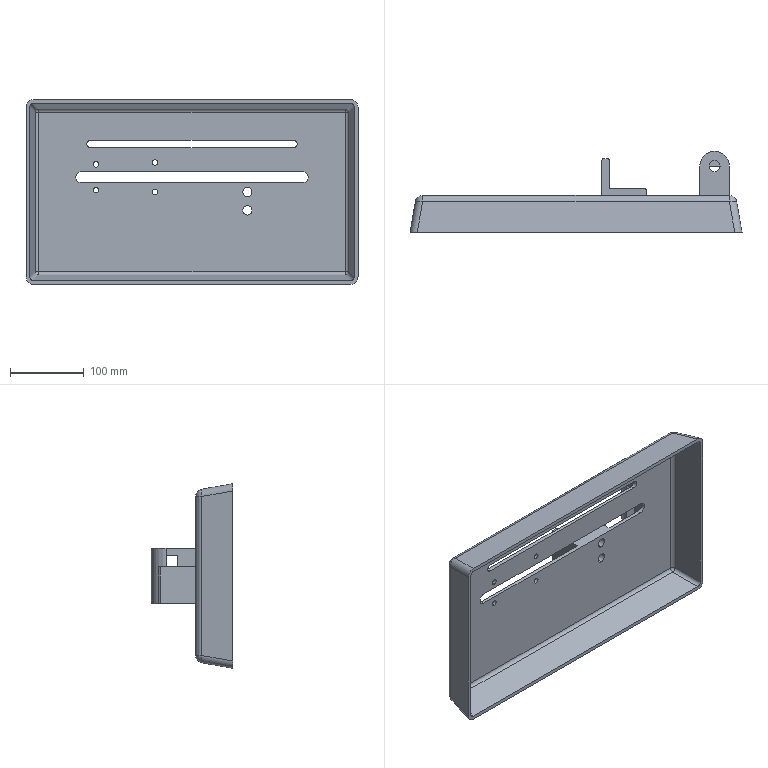Part | SolidWorks | features ICE 8, HoleWzd 4, Fillet 3, Extrusion 1 | 1 solid | 82 faces | box 450 x 110 x 250 mm | volume 893296 mm3 | cylinder 40 | plane 34 | sphere 8 | commonest cylinder face diameters 10 x10 7.5 x8 20 x8 15 x6 12.5 x4 5 x3